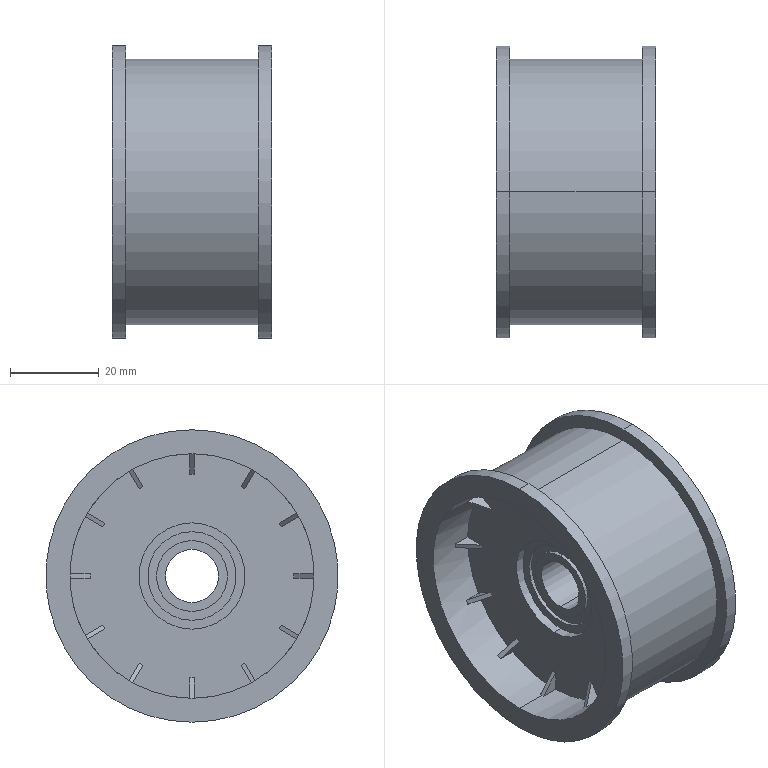Part | SolidWorks | features BaseBody 1 | 1 solid | 112 faces | box 36 x 66 x 66 mm | volume 49785 mm3 | plane 84 | cylinder 28 | commonest cylinder face diameters 12 x6 16 x4 20 x4 24 x4 55.2 x4 66 x4